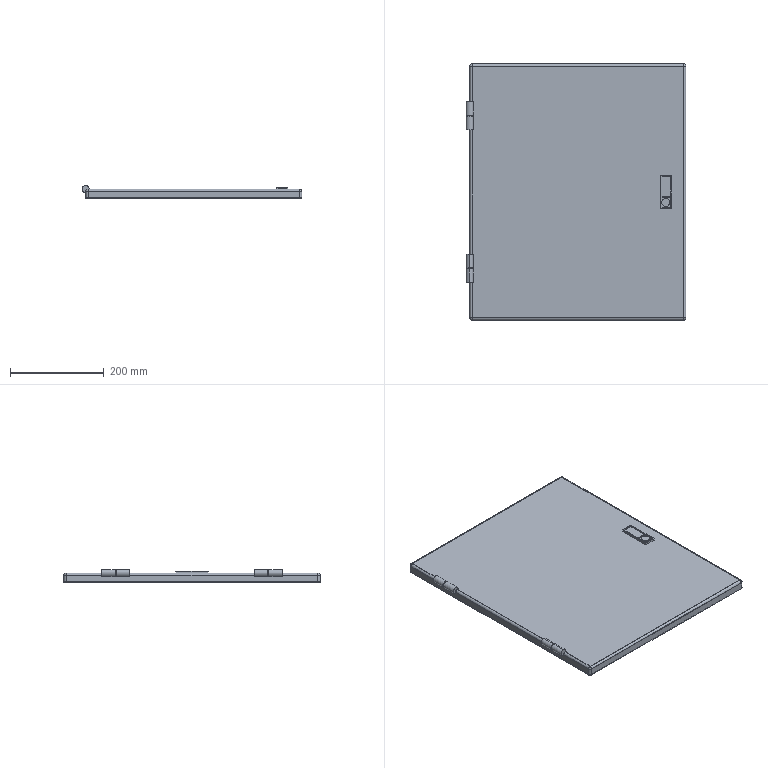Part | SolidWorks | features Cut 4, Boss 3, Extrusion 1, Fillet 1, LibraryFeature 1, MirrorPattern 1, Shell 1 | 1 solid | 88 faces | box 467.5 x 545 x 27.5 mm | volume 335829 mm3 | plane 44 | cylinder 36 | sphere 8 | commonest cylinder face diameters 15 x14 8 x10 10 x10 17 x2